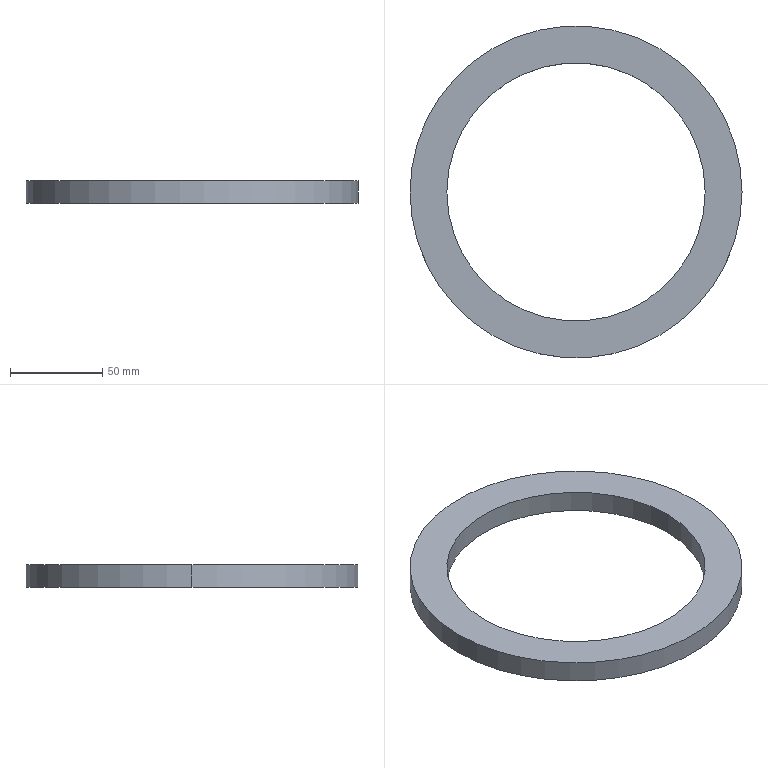Part | NX | features BREP 1 | 1 solid | 6 faces | box 180 x 180 x 12 mm | volume 120637 mm3 | cylinder 4 | plane 2 | commonest cylinder face diameters 140 x2 180 x2
STEP:
#1=CARTESIAN_POINT('',(-70.,0.,12.));
#2=VERTEX_POINT('',#1);
#3=CARTESIAN_POINT('',(70.,0.,12.));
#4=VERTEX_POINT('',#3);
#5=CARTESIAN_POINT('',(0.,0.,12.));
#6=DIRECTION('',(0.,0.,1.));
#7=DIRECTION('',(1.,0.,0.));
#8=AXIS2_PLACEMENT_3D('',#5,#6,#7);
#9=CIRCLE('',#8,70.);
#10=EDGE_CURVE('',#2,#4,#9,.T.);
#11=ORIENTED_EDGE('',*,*,#10,.T.);
#12=CARTESIAN_POINT('',(70.,0.,0.));
#13=VERTEX_POINT('',#12);
#14=CARTESIAN_POINT('',(70.,0.,12.));
#15=DIRECTION('',(0.,0.,-1.));
#16=VECTOR('',#15,1000.);
#17=LINE('',#14,#16);
#18=EDGE_CURVE('',#13,#4,#17,.F.);
#19=ORIENTED_EDGE('',*,*,#18,.F.);
#20=CARTESIAN_POINT('',(-70.,0.,0.));
#21=VERTEX_POINT('',#20);
#22=CARTESIAN_POINT('',(0.,0.,0.));
#23=DIRECTION('',(0.,0.,1.));
#24=DIRECTION('',(1.,0.,0.));
#25=AXIS2_PLACEMENT_3D('',#22,#23,#24);
#26=CIRCLE('',#25,70.);
#27=EDGE_CURVE('',#21,#13,#26,.T.);
#28=ORIENTED_EDGE('',*,*,#27,.F.);
#29=CARTESIAN_POINT('',(-70.,0.,12.));
#30=DIRECTION('',(0.,0.,-1.));
#31=VECTOR('',#30,1000.);
#32=LINE('',#29,#31);
#33=EDGE_CURVE('',#21,#2,#32,.F.);
#34=ORIENTED_EDGE('',*,*,#33,.T.);
#35=EDGE_LOOP('',(#11,#19,#28,#34));
#36=FACE_BOUND('',#35,.T.);
#37=CARTESIAN_POINT('',(0.,0.,12.));
#38=DIRECTION('',(0.,0.,-1.));
#39=DIRECTION('',(1.,0.,0.));
#40=AXIS2_PLACEMENT_3D('',#37,#38,#39);
#41=CYLINDRICAL_SURFACE('',#40,70.);
#42=ADVANCED_FACE('',(#36),#41,.F.);
#43=CARTESIAN_POINT('',(90.,0.,12.));
#44=VERTEX_POINT('',#43);
#45=CARTESIAN_POINT('',(-90.,0.,12.));
#46=VERTEX_POINT('',#45);
#47=CARTESIAN_POINT('',(0.,0.,12.));
#48=DIRECTION('',(0.,0.,1.));
#49=DIRECTION('',(1.,0.,0.));
#50=AXIS2_PLACEMENT_3D('',#47,#48,#49);
#51=CIRCLE('',#50,90.);
#52=EDGE_CURVE('',#44,#46,#51,.T.);
#53=ORIENTED_EDGE('',*,*,#52,.F.);
#54=CARTESIAN_POINT('',(90.,0.,0.));
#55=VERTEX_POINT('',#54);
#56=CARTESIAN_POINT('',(90.,0.,12.));
#57=DIRECTION('',(0.,0.,-1.));
#58=VECTOR('',#57,1000.);
#59=LINE('',#56,#58);
#60=EDGE_CURVE('',#55,#44,#59,.F.);
#61=ORIENTED_EDGE('',*,*,#60,.F.);
#62=CARTESIAN_POINT('',(-90.,0.,0.));
#63=VERTEX_POINT('',#62);
#64=CARTESIAN_POINT('',(0.,0.,0.));
#65=DIRECTION('',(0.,0.,1.));
#66=DIRECTION('',(1.,0.,0.));
#67=AXIS2_PLACEMENT_3D('',#64,#65,#66);
#68=CIRCLE('',#67,90.);
#69=EDGE_CURVE('',#55,#63,#68,.T.);
#70=ORIENTED_EDGE('',*,*,#69,.T.);
#71=CARTESIAN_POINT('',(-90.,0.,12.));
#72=DIRECTION('',(0.,0.,-1.));
#73=VECTOR('',#72,1000.);
#74=LINE('',#71,#73);
#75=EDGE_CURVE('',#63,#46,#74,.F.);
#76=ORIENTED_EDGE('',*,*,#75,.T.);
#77=EDGE_LOOP('',(#53,#61,#70,#76));
#78=FACE_BOUND('',#77,.T.);
#79=CARTESIAN_POINT('',(0.,0.,12.));
#80=DIRECTION('',(0.,0.,-1.));
#81=DIRECTION('',(1.,0.,0.));
#82=AXIS2_PLACEMENT_3D('',#79,#80,#81);
#83=CYLINDRICAL_SURFACE('',#82,90.);
#84=ADVANCED_FACE('',(#78),#83,.T.);
#85=CARTESIAN_POINT('',(0.,0.,12.));
#86=DIRECTION('',(0.,0.,1.));
#87=DIRECTION('',(1.,0.,0.));
#88=AXIS2_PLACEMENT_3D('',#85,#86,#87);
#89=CIRCLE('',#88,90.);
#90=EDGE_CURVE('',#46,#44,#89,.T.);
#91=ORIENTED_EDGE('',*,*,#90,.T.);
#92=ORIENTED_EDGE('',*,*,#52,.T.);
#93=EDGE_LOOP('',(#91,#92));
#94=FACE_BOUND('',#93,.T.);
#95=ORIENTED_EDGE('',*,*,#10,.F.);
#96=CARTESIAN_POINT('',(0.,0.,12.));
#97=DIRECTION('',(0.,0.,1.));
#98=DIRECTION('',(1.,0.,0.));
#99=AXIS2_PLACEMENT_3D('',#96,#97,#98);
#100=CIRCLE('',#99,70.);
#101=EDGE_CURVE('',#4,#2,#100,.T.);
#102=ORIENTED_EDGE('',*,*,#101,.F.);
#103=EDGE_LOOP('',(#95,#102));
#104=FACE_BOUND('',#103,.T.);
#105=CARTESIAN_POINT('',(0.,0.,12.));
#106=DIRECTION('',(0.,0.,1.));
#107=DIRECTION('',(-1.,0.,0.));
#108=AXIS2_PLACEMENT_3D('',#105,#106,#107);
#109=PLANE('',#108);
#110=ADVANCED_FACE('',(#94,#104),#109,.T.);
#111=CARTESIAN_POINT('',(0.,0.,0.));
#112=DIRECTION('',(0.,0.,1.));
#113=DIRECTION('',(1.,0.,0.));
#114=AXIS2_PLACEMENT_3D('',#111,#112,#113);
#115=CIRCLE('',#114,90.);
#116=EDGE_CURVE('',#63,#55,#115,.T.);
#117=ORIENTED_EDGE('',*,*,#116,.F.);
#118=ORIENTED_EDGE('',*,*,#69,.F.);
#119=EDGE_LOOP('',(#117,#118));
#120=FACE_BOUND('',#119,.T.);
#121=ORIENTED_EDGE('',*,*,#27,.T.);
#122=CARTESIAN_POINT('',(0.,0.,0.));
#123=DIRECTION('',(0.,0.,1.));
#124=DIRECTION('',(1.,0.,0.));
#125=AXIS2_PLACEMENT_3D('',#122,#123,#124);
#126=CIRCLE('',#125,70.);
#127=EDGE_CURVE('',#13,#21,#126,.T.);
#128=ORIENTED_EDGE('',*,*,#127,.T.);
#129=EDGE_LOOP('',(#121,#128));
#130=FACE_BOUND('',#129,.T.);
#131=CARTESIAN_POINT('',(0.,0.,0.));
#132=DIRECTION('',(0.,0.,1.));
#133=DIRECTION('',(-1.,0.,0.));
#134=AXIS2_PLACEMENT_3D('',#131,#132,#133);
#135=PLANE('',#134);
#136=ADVANCED_FACE('',(#120,#130),#135,.F.);
#137=ORIENTED_EDGE('',*,*,#60,.T.);
#138=ORIENTED_EDGE('',*,*,#90,.F.);
#139=ORIENTED_EDGE('',*,*,#75,.F.);
#140=ORIENTED_EDGE('',*,*,#116,.T.);
#141=EDGE_LOOP('',(#137,#138,#139,#140));
#142=FACE_BOUND('',#141,.T.);
#143=CARTESIAN_POINT('',(0.,0.,12.));
#144=DIRECTION('',(0.,0.,-1.));
#145=DIRECTION('',(1.,0.,0.));
#146=AXIS2_PLACEMENT_3D('',#143,#144,#145);
#147=CYLINDRICAL_SURFACE('',#146,90.);
#148=ADVANCED_FACE('',(#142),#147,.T.);
#149=ORIENTED_EDGE('',*,*,#18,.T.);
#150=ORIENTED_EDGE('',*,*,#101,.T.);
#151=ORIENTED_EDGE('',*,*,#33,.F.);
#152=ORIENTED_EDGE('',*,*,#127,.F.);
#153=EDGE_LOOP('',(#149,#150,#151,#152));
#154=FACE_BOUND('',#153,.T.);
#155=CARTESIAN_POINT('',(0.,0.,12.));
#156=DIRECTION('',(0.,0.,-1.));
#157=DIRECTION('',(1.,0.,0.));
#158=AXIS2_PLACEMENT_3D('',#155,#156,#157);
#159=CYLINDRICAL_SURFACE('',#158,70.);
#160=ADVANCED_FACE('',(#154),#159,.F.);
#161=CLOSED_SHELL('',(#42,#84,#110,#136,#148,#160));
#162=MANIFOLD_SOLID_BREP('',#161);
#163=(LENGTH_UNIT()NAMED_UNIT(*)SI_UNIT(.MILLI.,.METRE.));
#164=UNCERTAINTY_MEASURE_WITH_UNIT(LENGTH_MEASURE(0.00001),#163,'','');
#165=(NAMED_UNIT(*)PLANE_ANGLE_UNIT()SI_UNIT($,.RADIAN.));
#166=(NAMED_UNIT(*)SI_UNIT($,.STERADIAN.)SOLID_ANGLE_UNIT());
#167=(GEOMETRIC_REPRESENTATION_CONTEXT(3)GLOBAL_UNCERTAINTY_ASSIGNED_CONTEXT((#164))GLOBAL_UNIT_ASSIGNED_CONTEXT((#163,#165,#166))REPRESENTATION_CONTEXT('',''));
#168=ADVANCED_BREP_SHAPE_REPRESENTATION('',(#162),#167);